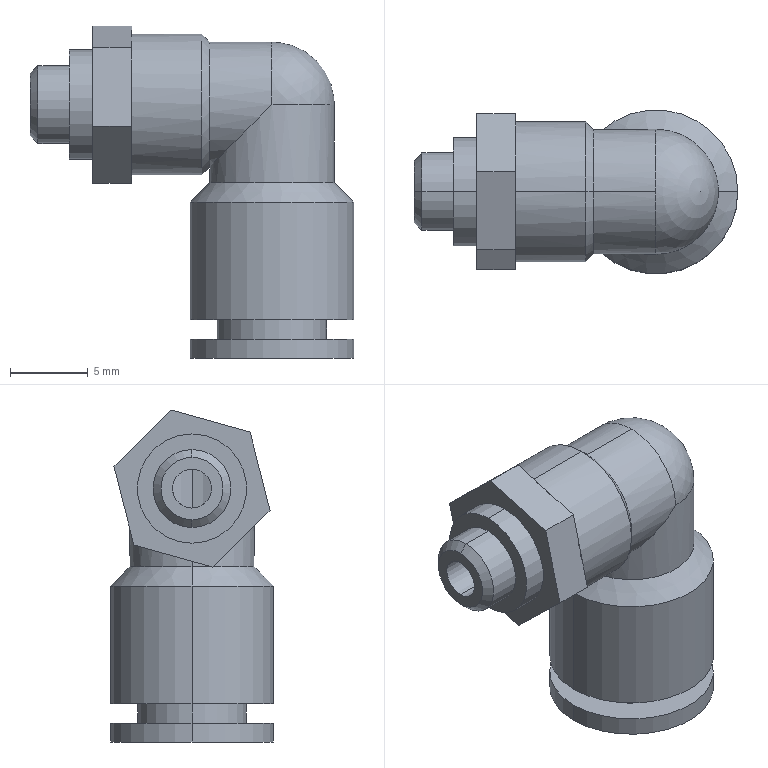Part | SolidWorks | features ICE 10, Chamfer 3, Extrusion 1, RevCut 1, Sweep 1 | 2 solids | 50 faces | box 20.75 x 10.5 x 21.285 mm | volume 1349 mm3 | cylinder 22 | plane 21 | cone 6 | sphere 1 | commonest cylinder face diameters 2.5 x4 7 x4 8 x4 10.5 x4 5 x2 6 x2
STEP:
#1=CARTESIAN_POINT('',(-4.,0.,15.));
#2=VERTEX_POINT('',#1);
#3=CARTESIAN_POINT('',(-4.,0.,17.5));
#4=VERTEX_POINT('',#3);
#5=CARTESIAN_POINT('',(-4.,0.,16.25));
#6=DIRECTION('',(-1.,0.,0.));
#7=DIRECTION('',(0.,0.,1.));
#8=AXIS2_PLACEMENT_3D('',#5,#6,#7);
#9=CIRCLE('',#8,1.25);
#10=EDGE_CURVE('',#2,#4,#9,.T.);
#11=ORIENTED_EDGE('',*,*,#10,.F.);
#12=CARTESIAN_POINT('',(-15.5,0.,15.));
#13=VERTEX_POINT('',#12);
#14=CARTESIAN_POINT('',(2.5,0.,15.));
#15=DIRECTION('',(-1.,0.,0.));
#16=VECTOR('',#15,1000.);
#17=LINE('',#14,#16);
#18=EDGE_CURVE('',#2,#13,#17,.T.);
#19=ORIENTED_EDGE('',*,*,#18,.T.);
#20=CARTESIAN_POINT('',(-15.5,0.,17.5));
#21=VERTEX_POINT('',#20);
#22=CARTESIAN_POINT('',(-15.5,0.,16.25));
#23=DIRECTION('',(-1.,0.,0.));
#24=DIRECTION('',(0.,0.,1.));
#25=AXIS2_PLACEMENT_3D('',#22,#23,#24);
#26=CIRCLE('',#25,1.25);
#27=EDGE_CURVE('',#13,#21,#26,.T.);
#28=ORIENTED_EDGE('',*,*,#27,.T.);
#29=CARTESIAN_POINT('',(2.5,0.,17.5));
#30=DIRECTION('',(-1.,0.,0.));
#31=VECTOR('',#30,1000.);
#32=LINE('',#29,#31);
#33=EDGE_CURVE('',#4,#21,#32,.T.);
#34=ORIENTED_EDGE('',*,*,#33,.F.);
#35=EDGE_LOOP('',(#11,#19,#28,#34));
#36=FACE_OUTER_BOUND('',#35,.T.);
#37=CARTESIAN_POINT('',(2.5,0.,16.25));
#38=DIRECTION('',(-1.,0.,0.));
#39=DIRECTION('',(0.,0.,1.));
#40=AXIS2_PLACEMENT_3D('',#37,#38,#39);
#41=CYLINDRICAL_SURFACE('',#40,1.25);
#42=ADVANCED_FACE('',(#36),#41,.F.);
#43=CARTESIAN_POINT('',(-15.5,0.,18.25));
#44=VERTEX_POINT('',#43);
#45=CARTESIAN_POINT('',(-15.5,0.,14.25));
#46=VERTEX_POINT('',#45);
#47=CARTESIAN_POINT('',(-15.5,0.,16.25));
#48=DIRECTION('',(-1.,0.,0.));
#49=DIRECTION('',(0.,0.,1.));
#50=AXIS2_PLACEMENT_3D('',#47,#48,#49);
#51=CIRCLE('',#50,2.);
#52=EDGE_CURVE('',#44,#46,#51,.T.);
#53=ORIENTED_EDGE('',*,*,#52,.F.);
#54=CARTESIAN_POINT('',(-15.,0.,18.75));
#55=VERTEX_POINT('',#54);
#56=CARTESIAN_POINT('',(-15.5,0.,18.25));
#57=DIRECTION('',(0.7071,0.,0.7071));
#58=VECTOR('',#57,1000.);
#59=LINE('',#56,#58);
#60=EDGE_CURVE('',#44,#55,#59,.T.);
#61=ORIENTED_EDGE('',*,*,#60,.T.);
#62=CARTESIAN_POINT('',(-15.,0.,13.75));
#63=VERTEX_POINT('',#62);
#64=CARTESIAN_POINT('',(-15.,0.,16.25));
#65=DIRECTION('',(1.,0.,0.));
#66=DIRECTION('',(0.,0.,1.));
#67=AXIS2_PLACEMENT_3D('',#64,#65,#66);
#68=CIRCLE('',#67,2.5);
#69=EDGE_CURVE('',#63,#55,#68,.T.);
#70=ORIENTED_EDGE('',*,*,#69,.F.);
#71=CARTESIAN_POINT('',(-15.5,0.,14.25));
#72=DIRECTION('',(0.7071,0.,-0.7071));
#73=VECTOR('',#72,1000.);
#74=LINE('',#71,#73);
#75=EDGE_CURVE('',#46,#63,#74,.T.);
#76=ORIENTED_EDGE('',*,*,#75,.F.);
#77=EDGE_LOOP('',(#53,#61,#70,#76));
#78=FACE_OUTER_BOUND('',#77,.T.);
#79=CARTESIAN_POINT('',(-15.5,0.,16.25));
#80=DIRECTION('',(1.,0.,0.));
#81=DIRECTION('',(0.,0.,-1.));
#82=AXIS2_PLACEMENT_3D('',#79,#80,#81);
#83=CONICAL_SURFACE('',#82,2.,0.7854);
#84=ADVANCED_FACE('',(#78),#83,.T.);
#85=ORIENTED_EDGE('',*,*,#69,.T.);
#86=CARTESIAN_POINT('',(-13.,0.,18.75));
#87=VERTEX_POINT('',#86);
#88=CARTESIAN_POINT('',(-15.5,0.,18.75));
#89=DIRECTION('',(1.,0.,0.));
#90=VECTOR('',#89,1000.);
#91=LINE('',#88,#90);
#92=EDGE_CURVE('',#55,#87,#91,.T.);
#93=ORIENTED_EDGE('',*,*,#92,.T.);
#94=CARTESIAN_POINT('',(-13.,0.,13.75));
#95=VERTEX_POINT('',#94);
#96=CARTESIAN_POINT('',(-13.,0.,16.25));
#97=DIRECTION('',(-1.,0.,0.));
#98=DIRECTION('',(0.,0.,1.));
#99=AXIS2_PLACEMENT_3D('',#96,#97,#98);
#100=CIRCLE('',#99,2.5);
#101=EDGE_CURVE('',#87,#95,#100,.T.);
#102=ORIENTED_EDGE('',*,*,#101,.T.);
#103=CARTESIAN_POINT('',(-15.5,0.,13.75));
#104=DIRECTION('',(1.,0.,0.));
#105=VECTOR('',#104,1000.);
#106=LINE('',#103,#105);
#107=EDGE_CURVE('',#63,#95,#106,.T.);
#108=ORIENTED_EDGE('',*,*,#107,.F.);
#109=EDGE_LOOP('',(#85,#93,#102,#108));
#110=FACE_OUTER_BOUND('',#109,.T.);
#111=CARTESIAN_POINT('',(-15.5,0.,16.25));
#112=DIRECTION('',(1.,0.,0.));
#113=DIRECTION('',(0.,0.,-1.));
#114=AXIS2_PLACEMENT_3D('',#111,#112,#113);
#115=CYLINDRICAL_SURFACE('',#114,2.5);
#116=ADVANCED_FACE('',(#110),#115,.T.);
#117=CARTESIAN_POINT('',(-13.,0.,19.75));
#118=VERTEX_POINT('',#117);
#119=CARTESIAN_POINT('',(-13.,0.,12.75));
#120=VERTEX_POINT('',#119);
#121=CARTESIAN_POINT('',(-13.,0.,16.25));
#122=DIRECTION('',(-1.,0.,0.));
#123=DIRECTION('',(0.,0.,1.));
#124=AXIS2_PLACEMENT_3D('',#121,#122,#123);
#125=CIRCLE('',#124,3.5);
#126=EDGE_CURVE('',#118,#120,#125,.T.);
#127=ORIENTED_EDGE('',*,*,#126,.F.);
#128=CARTESIAN_POINT('',(-11.5,0.,19.75));
#129=VERTEX_POINT('',#128);
#130=CARTESIAN_POINT('',(-13.,0.,19.75));
#131=DIRECTION('',(1.,0.,0.));
#132=VECTOR('',#131,1000.);
#133=LINE('',#130,#132);
#134=EDGE_CURVE('',#118,#129,#133,.T.);
#135=ORIENTED_EDGE('',*,*,#134,.T.);
#136=CARTESIAN_POINT('',(-11.5,0.,12.75));
#137=VERTEX_POINT('',#136);
#138=CARTESIAN_POINT('',(-11.5,0.,16.25));
#139=DIRECTION('',(-1.,0.,0.));
#140=DIRECTION('',(0.,0.,1.));
#141=AXIS2_PLACEMENT_3D('',#138,#139,#140);
#142=CIRCLE('',#141,3.5);
#143=EDGE_CURVE('',#129,#137,#142,.T.);
#144=ORIENTED_EDGE('',*,*,#143,.T.);
#145=CARTESIAN_POINT('',(-13.,0.,12.75));
#146=DIRECTION('',(1.,0.,0.));
#147=VECTOR('',#146,1000.);
#148=LINE('',#145,#147);
#149=EDGE_CURVE('',#120,#137,#148,.T.);
#150=ORIENTED_EDGE('',*,*,#149,.F.);
#151=EDGE_LOOP('',(#127,#135,#144,#150));
#152=FACE_OUTER_BOUND('',#151,.T.);
#153=CARTESIAN_POINT('',(-13.,0.,16.25));
#154=DIRECTION('',(1.,0.,0.));
#155=DIRECTION('',(0.,0.,-1.));
#156=AXIS2_PLACEMENT_3D('',#153,#154,#155);
#157=CYLINDRICAL_SURFACE('',#156,3.5);
#158=ADVANCED_FACE('',(#152),#157,.T.);
#159=CARTESIAN_POINT('',(-4.,0.,12.25));
#160=VERTEX_POINT('',#159);
#161=CARTESIAN_POINT('',(-4.,0.,20.25));
#162=VERTEX_POINT('',#161);
#163=CARTESIAN_POINT('',(-4.,0.,16.25));
#164=DIRECTION('',(1.,0.,0.));
#165=DIRECTION('',(0.,0.,1.));
#166=AXIS2_PLACEMENT_3D('',#163,#164,#165);
#167=CIRCLE('',#166,4.);
#168=EDGE_CURVE('',#160,#162,#167,.T.);
#169=ORIENTED_EDGE('',*,*,#168,.F.);
#170=CARTESIAN_POINT('',(-4.5,0.,11.75));
#171=VERTEX_POINT('',#170);
#172=CARTESIAN_POINT('',(-4.5,0.,11.75));
#173=DIRECTION('',(-0.7071,0.,-0.7071));
#174=VECTOR('',#173,1000.);
#175=LINE('',#172,#174);
#176=EDGE_CURVE('',#160,#171,#175,.T.);
#177=ORIENTED_EDGE('',*,*,#176,.T.);
#178=CARTESIAN_POINT('',(-4.5,0.,20.75));
#179=VERTEX_POINT('',#178);
#180=CARTESIAN_POINT('',(-4.5,0.,16.25));
#181=DIRECTION('',(-1.,0.,0.));
#182=DIRECTION('',(0.,0.,1.));
#183=AXIS2_PLACEMENT_3D('',#180,#181,#182);
#184=CIRCLE('',#183,4.5);
#185=EDGE_CURVE('',#179,#171,#184,.T.);
#186=ORIENTED_EDGE('',*,*,#185,.F.);
#187=CARTESIAN_POINT('',(-4.5,0.,20.75));
#188=DIRECTION('',(-0.7071,0.,0.7071));
#189=VECTOR('',#188,1000.);
#190=LINE('',#187,#189);
#191=EDGE_CURVE('',#162,#179,#190,.T.);
#192=ORIENTED_EDGE('',*,*,#191,.F.);
#193=EDGE_LOOP('',(#169,#177,#186,#192));
#194=FACE_OUTER_BOUND('',#193,.T.);
#195=CARTESIAN_POINT('',(-4.5,0.,16.25));
#196=DIRECTION('',(-1.,0.,0.));
#197=DIRECTION('',(0.,0.,1.));
#198=AXIS2_PLACEMENT_3D('',#195,#196,#197);
#199=CONICAL_SURFACE('',#198,4.5,0.7854);
#200=ADVANCED_FACE('',(#194),#199,.T.);
#201=CARTESIAN_POINT('',(-9.,0.,20.75));
#202=VERTEX_POINT('',#201);
#203=CARTESIAN_POINT('',(-9.,3.143,19.47));
#204=VERTEX_POINT('',#203);
#205=CARTESIAN_POINT('',(-9.,0.,16.25));
#206=DIRECTION('',(-1.,0.,0.));
#207=DIRECTION('',(0.,0.,1.));
#208=AXIS2_PLACEMENT_3D('',#205,#206,#207);
#209=CIRCLE('',#208,4.5);
#210=EDGE_CURVE('',#202,#204,#209,.T.);
#211=ORIENTED_EDGE('',*,*,#210,.F.);
#212=CARTESIAN_POINT('',(-9.,0.,20.75));
#213=DIRECTION('',(1.,0.,0.));
#214=VECTOR('',#213,1000.);
#215=LINE('',#212,#214);
#216=EDGE_CURVE('',#202,#179,#215,.T.);
#217=ORIENTED_EDGE('',*,*,#216,.T.);
#218=ORIENTED_EDGE('',*,*,#185,.T.);
#219=CARTESIAN_POINT('',(-9.,0.,11.75));
#220=VERTEX_POINT('',#219);
#221=CARTESIAN_POINT('',(-9.,0.,11.75));
#222=DIRECTION('',(1.,0.,0.));
#223=VECTOR('',#222,1000.);
#224=LINE('',#221,#223);
#225=EDGE_CURVE('',#220,#171,#224,.T.);
#226=ORIENTED_EDGE('',*,*,#225,.F.);
#227=CARTESIAN_POINT('',(-9.,1.217,11.918));
#228=VERTEX_POINT('',#227);
#229=CARTESIAN_POINT('',(-9.,0.,16.25));
#230=DIRECTION('',(-1.,0.,0.));
#231=DIRECTION('',(0.,0.,1.));
#232=AXIS2_PLACEMENT_3D('',#229,#230,#231);
#233=CIRCLE('',#232,4.5);
#234=EDGE_CURVE('',#228,#220,#233,.T.);
#235=ORIENTED_EDGE('',*,*,#234,.F.);
#236=CARTESIAN_POINT('',(-9.,4.36,15.138));
#237=VERTEX_POINT('',#236);
#238=CARTESIAN_POINT('',(-9.,0.,16.25));
#239=DIRECTION('',(-1.,0.,0.));
#240=DIRECTION('',(0.,0.,1.));
#241=AXIS2_PLACEMENT_3D('',#238,#239,#240);
#242=CIRCLE('',#241,4.5);
#243=EDGE_CURVE('',#237,#228,#242,.T.);
#244=ORIENTED_EDGE('',*,*,#243,.F.);
#245=CARTESIAN_POINT('',(-9.,0.,16.25));
#246=DIRECTION('',(-1.,0.,0.));
#247=DIRECTION('',(0.,0.,1.));
#248=AXIS2_PLACEMENT_3D('',#245,#246,#247);
#249=CIRCLE('',#248,4.5);
#250=EDGE_CURVE('',#204,#237,#249,.T.);
#251=ORIENTED_EDGE('',*,*,#250,.F.);
#252=EDGE_LOOP('',(#211,#217,#218,#226,#235,#244,#251));
#253=FACE_OUTER_BOUND('',#252,.T.);
#254=CARTESIAN_POINT('',(-9.,0.,16.25));
#255=DIRECTION('',(1.,0.,0.));
#256=DIRECTION('',(0.,0.,-1.));
#257=AXIS2_PLACEMENT_3D('',#254,#255,#256);
#258=CYLINDRICAL_SURFACE('',#257,4.5);
#259=ADVANCED_FACE('',(#253),#258,.T.);
#260=CARTESIAN_POINT('',(-13.,0.,16.25));
#261=DIRECTION('',(-1.,0.,0.));
#262=DIRECTION('',(0.,0.,1.));
#263=AXIS2_PLACEMENT_3D('',#260,#261,#262);
#264=CIRCLE('',#263,3.5);
#265=EDGE_CURVE('',#120,#118,#264,.T.);
#266=ORIENTED_EDGE('',*,*,#265,.T.);
#267=ORIENTED_EDGE('',*,*,#126,.T.);
#268=EDGE_LOOP('',(#266,#267));
#269=FACE_OUTER_BOUND('',#268,.T.);
#270=CARTESIAN_POINT('',(-13.,0.,16.25));
#271=DIRECTION('',(-1.,0.,0.));
#272=DIRECTION('',(0.,0.,1.));
#273=AXIS2_PLACEMENT_3D('',#270,#271,#272);
#274=CIRCLE('',#273,2.5);
#275=EDGE_CURVE('',#95,#87,#274,.T.);
#276=ORIENTED_EDGE('',*,*,#275,.F.);
#277=ORIENTED_EDGE('',*,*,#101,.F.);
#278=EDGE_LOOP('',(#276,#277));
#279=FACE_BOUND('',#278,.T.);
#280=CARTESIAN_POINT('',(-13.,0.,16.25));
#281=DIRECTION('',(-1.,0.,0.));
#282=DIRECTION('',(0.,0.,1.));
#283=AXIS2_PLACEMENT_3D('',#280,#281,#282);
#284=PLANE('',#283);
#285=ADVANCED_FACE('',(#269,#279),#284,.T.);
#286=CARTESIAN_POINT('',(-11.5,-3.718,19.88));
#287=VERTEX_POINT('',#286);
#288=CARTESIAN_POINT('',(-11.5,1.284,21.285));
#289=VERTEX_POINT('',#288);
#290=CARTESIAN_POINT('',(-11.5,-3.718,19.88));
#291=DIRECTION('',(0.,0.9627,0.2704));
#292=VECTOR('',#291,1000.);
#293=LINE('',#290,#292);
#294=EDGE_CURVE('',#287,#289,#293,.T.);
#295=ORIENTED_EDGE('',*,*,#294,.T.);
#296=CARTESIAN_POINT('',(-11.5,5.003,17.655));
#297=VERTEX_POINT('',#296);
#298=CARTESIAN_POINT('',(-11.5,1.284,21.285));
#299=DIRECTION('',(0.,0.7156,-0.6985));
#300=VECTOR('',#299,1000.);
#301=LINE('',#298,#300);
#302=EDGE_CURVE('',#289,#297,#301,.T.);
#303=ORIENTED_EDGE('',*,*,#302,.T.);
#304=CARTESIAN_POINT('',(-11.5,3.718,12.62));
#305=VERTEX_POINT('',#304);
#306=CARTESIAN_POINT('',(-11.5,5.003,17.655));
#307=DIRECTION('',(0.,-0.2472,-0.969));
#308=VECTOR('',#307,1000.);
#309=LINE('',#306,#308);
#310=EDGE_CURVE('',#297,#305,#309,.T.);
#311=ORIENTED_EDGE('',*,*,#310,.T.);
#312=CARTESIAN_POINT('',(-11.5,-1.284,11.215));
#313=VERTEX_POINT('',#312);
#314=CARTESIAN_POINT('',(-11.5,3.718,12.62));
#315=DIRECTION('',(0.,-0.9627,-0.2704));
#316=VECTOR('',#315,1000.);
#317=LINE('',#314,#316);
#318=EDGE_CURVE('',#305,#313,#317,.T.);
#319=ORIENTED_EDGE('',*,*,#318,.T.);
#320=CARTESIAN_POINT('',(-11.5,-5.003,14.845));
#321=VERTEX_POINT('',#320);
#322=CARTESIAN_POINT('',(-11.5,-1.284,11.215));
#323=DIRECTION('',(0.,-0.7156,0.6985));
#324=VECTOR('',#323,1000.);
#325=LINE('',#322,#324);
#326=EDGE_CURVE('',#313,#321,#325,.T.);
#327=ORIENTED_EDGE('',*,*,#326,.T.);
#328=CARTESIAN_POINT('',(-11.5,-5.003,14.845));
#329=DIRECTION('',(0.,0.2472,0.969));
#330=VECTOR('',#329,1000.);
#331=LINE('',#328,#330);
#332=EDGE_CURVE('',#321,#287,#331,.T.);
#333=ORIENTED_EDGE('',*,*,#332,.T.);
#334=EDGE_LOOP('',(#295,#303,#311,#319,#327,#333));
#335=FACE_OUTER_BOUND('',#334,.T.);
#336=CARTESIAN_POINT('',(-11.5,0.,16.25));
#337=DIRECTION('',(-1.,0.,0.));
#338=DIRECTION('',(0.,0.,1.));
#339=AXIS2_PLACEMENT_3D('',#336,#337,#338);
#340=CIRCLE('',#339,3.5);
#341=EDGE_CURVE('',#137,#129,#340,.T.);
#342=ORIENTED_EDGE('',*,*,#341,.F.);
#343=ORIENTED_EDGE('',*,*,#143,.F.);
#344=EDGE_LOOP('',(#342,#343));
#345=FACE_BOUND('',#344,.T.);
#346=CARTESIAN_POINT('',(-11.5,0.,0.));
#347=DIRECTION('',(-1.,0.,0.));
#348=DIRECTION('',(0.,0.,1.));
#349=AXIS2_PLACEMENT_3D('',#346,#347,#348);
#350=PLANE('',#349);
#351=ADVANCED_FACE('',(#335,#345),#350,.T.);
#352=ORIENTED_EDGE('',*,*,#216,.F.);
#353=CARTESIAN_POINT('',(-9.,-1.217,20.582));
#354=VERTEX_POINT('',#353);
#355=CARTESIAN_POINT('',(-9.,0.,16.25));
#356=DIRECTION('',(-1.,0.,0.));
#357=DIRECTION('',(0.,0.,1.));
#358=AXIS2_PLACEMENT_3D('',#355,#356,#357);
#359=CIRCLE('',#358,4.5);
#360=EDGE_CURVE('',#354,#202,#359,.T.);
#361=ORIENTED_EDGE('',*,*,#360,.F.);
#362=CARTESIAN_POINT('',(-9.,-4.36,17.362));
#363=VERTEX_POINT('',#362);
#364=CARTESIAN_POINT('',(-9.,0.,16.25));
#365=DIRECTION('',(-1.,0.,0.));
#366=DIRECTION('',(0.,0.,1.));
#367=AXIS2_PLACEMENT_3D('',#364,#365,#366);
#368=CIRCLE('',#367,4.5);
#369=EDGE_CURVE('',#363,#354,#368,.T.);
#370=ORIENTED_EDGE('',*,*,#369,.F.);
#371=CARTESIAN_POINT('',(-9.,-3.143,13.03));
#372=VERTEX_POINT('',#371);
#373=CARTESIAN_POINT('',(-9.,0.,16.25));
#374=DIRECTION('',(-1.,0.,0.));
#375=DIRECTION('',(0.,0.,1.));
#376=AXIS2_PLACEMENT_3D('',#373,#374,#375);
#377=CIRCLE('',#376,4.5);
#378=EDGE_CURVE('',#372,#363,#377,.T.);
#379=ORIENTED_EDGE('',*,*,#378,.F.);
#380=CARTESIAN_POINT('',(-9.,0.,16.25));
#381=DIRECTION('',(-1.,0.,0.));
#382=DIRECTION('',(0.,0.,1.));
#383=AXIS2_PLACEMENT_3D('',#380,#381,#382);
#384=CIRCLE('',#383,4.5);
#385=EDGE_CURVE('',#220,#372,#384,.T.);
#386=ORIENTED_EDGE('',*,*,#385,.F.);
#387=ORIENTED_EDGE('',*,*,#225,.T.);
#388=CARTESIAN_POINT('',(-4.5,0.,16.25));
#389=DIRECTION('',(-1.,0.,0.));
#390=DIRECTION('',(0.,0.,1.));
#391=AXIS2_PLACEMENT_3D('',#388,#389,#390);
#392=CIRCLE('',#391,4.5);
#393=EDGE_CURVE('',#171,#179,#392,.T.);
#394=ORIENTED_EDGE('',*,*,#393,.T.);
#395=EDGE_LOOP('',(#352,#361,#370,#379,#386,#387,#394));
#396=FACE_OUTER_BOUND('',#395,.T.);
#397=CARTESIAN_POINT('',(-9.,0.,16.25));
#398=DIRECTION('',(1.,0.,0.));
#399=DIRECTION('',(0.,0.,-1.));
#400=AXIS2_PLACEMENT_3D('',#397,#398,#399);
#401=CYLINDRICAL_SURFACE('',#400,4.5);
#402=ADVANCED_FACE('',(#396),#401,.T.);
#403=CARTESIAN_POINT('',(-4.,0.,16.25));
#404=DIRECTION('',(-1.,0.,0.));
#405=DIRECTION('',(0.,0.,1.));
#406=AXIS2_PLACEMENT_3D('',#403,#404,#405);
#407=CIRCLE('',#406,1.25);
#408=EDGE_CURVE('',#4,#2,#407,.T.);
#409=ORIENTED_EDGE('',*,*,#408,.T.);
#410=ORIENTED_EDGE('',*,*,#10,.T.);
#411=EDGE_LOOP('',(#409,#410));
#412=FACE_BOUND('',#411,.T.);
#413=CARTESIAN_POINT('',(-4.,0.,16.25));
#414=DIRECTION('',(1.,0.,0.));
#415=DIRECTION('',(0.,0.,1.));
#416=AXIS2_PLACEMENT_3D('',#413,#414,#415);
#417=CIRCLE('',#416,4.);
#418=EDGE_CURVE('',#162,#160,#417,.T.);
#419=ORIENTED_EDGE('',*,*,#418,.T.);
#420=ORIENTED_EDGE('',*,*,#168,.T.);
#421=EDGE_LOOP('',(#419,#420));
#422=FACE_OUTER_BOUND('',#421,.T.);
#423=CARTESIAN_POINT('',(-4.,0.,16.25));
#424=DIRECTION('',(-1.,0.,0.));
#425=DIRECTION('',(0.,0.,1.));
#426=AXIS2_PLACEMENT_3D('',#423,#424,#425);
#427=PLANE('',#426);
#428=ADVANCED_FACE('',(#412,#422),#427,.F.);
#429=ORIENTED_EDGE('',*,*,#176,.F.);
#430=ORIENTED_EDGE('',*,*,#418,.F.);
#431=ORIENTED_EDGE('',*,*,#191,.T.);
#432=ORIENTED_EDGE('',*,*,#393,.F.);
#433=EDGE_LOOP('',(#429,#430,#431,#432));
#434=FACE_OUTER_BOUND('',#433,.T.);
#435=CARTESIAN_POINT('',(-4.5,0.,16.25));
#436=DIRECTION('',(-1.,0.,0.));
#437=DIRECTION('',(0.,0.,1.));
#438=AXIS2_PLACEMENT_3D('',#435,#436,#437);
#439=CONICAL_SURFACE('',#438,4.5,0.7854);
#440=ADVANCED_FACE('',(#434),#439,.T.);
#441=CARTESIAN_POINT('',(-9.,5.003,17.655));
#442=VERTEX_POINT('',#441);
#443=CARTESIAN_POINT('',(-9.,1.284,21.285));
#444=DIRECTION('',(0.,0.7156,-0.6985));
#445=VECTOR('',#444,1000.);
#446=LINE('',#443,#445);
#447=EDGE_CURVE('',#204,#442,#446,.T.);
#448=ORIENTED_EDGE('',*,*,#447,.F.);
#449=ORIENTED_EDGE('',*,*,#250,.T.);
#450=CARTESIAN_POINT('',(-9.,5.003,17.655));
#451=DIRECTION('',(0.,-0.2472,-0.969));
#452=VECTOR('',#451,1000.);
#453=LINE('',#450,#452);
#454=EDGE_CURVE('',#442,#237,#453,.T.);
#455=ORIENTED_EDGE('',*,*,#454,.F.);
#456=EDGE_LOOP('',(#448,#449,#455));
#457=FACE_OUTER_BOUND('',#456,.T.);
#458=CARTESIAN_POINT('',(-9.,0.,0.));
#459=DIRECTION('',(-1.,0.,0.));
#460=DIRECTION('',(0.,0.,1.));
#461=AXIS2_PLACEMENT_3D('',#458,#459,#460);
#462=PLANE('',#461);
#463=ADVANCED_FACE('',(#457),#462,.F.);
#464=CARTESIAN_POINT('',(-9.,3.718,12.62));
#465=VERTEX_POINT('',#464);
#466=CARTESIAN_POINT('',(-9.,5.003,17.655));
#467=DIRECTION('',(0.,-0.2472,-0.969));
#468=VECTOR('',#467,1000.);
#469=LINE('',#466,#468);
#470=EDGE_CURVE('',#237,#465,#469,.T.);
#471=ORIENTED_EDGE('',*,*,#470,.F.);
#472=ORIENTED_EDGE('',*,*,#243,.T.);
#473=CARTESIAN_POINT('',(-9.,3.718,12.62));
#474=DIRECTION('',(0.,-0.9627,-0.2704));
#475=VECTOR('',#474,1000.);
#476=LINE('',#473,#475);
#477=EDGE_CURVE('',#465,#228,#476,.T.);
#478=ORIENTED_EDGE('',*,*,#477,.F.);
#479=EDGE_LOOP('',(#471,#472,#478));
#480=FACE_OUTER_BOUND('',#479,.T.);
#481=CARTESIAN_POINT('',(-9.,0.,0.));
#482=DIRECTION('',(-1.,0.,0.));
#483=DIRECTION('',(0.,0.,1.));
#484=AXIS2_PLACEMENT_3D('',#481,#482,#483);
#485=PLANE('',#484);
#486=ADVANCED_FACE('',(#480),#485,.F.);
#487=CARTESIAN_POINT('',(-9.,-1.284,11.215));
#488=VERTEX_POINT('',#487);
#489=CARTESIAN_POINT('',(-9.,3.718,12.62));
#490=DIRECTION('',(0.,-0.9627,-0.2704));
#491=VECTOR('',#490,1000.);
#492=LINE('',#489,#491);
#493=EDGE_CURVE('',#228,#488,#492,.T.);
#494=ORIENTED_EDGE('',*,*,#493,.F.);
#495=ORIENTED_EDGE('',*,*,#234,.T.);
#496=ORIENTED_EDGE('',*,*,#385,.T.);
#497=CARTESIAN_POINT('',(-9.,-1.284,11.215));
#498=DIRECTION('',(0.,-0.7156,0.6985));
#499=VECTOR('',#498,1000.);
#500=LINE('',#497,#499);
#501=EDGE_CURVE('',#488,#372,#500,.T.);
#502=ORIENTED_EDGE('',*,*,#501,.F.);
#503=EDGE_LOOP('',(#494,#495,#496,#502));
#504=FACE_OUTER_BOUND('',#503,.T.);
#505=CARTESIAN_POINT('',(-9.,0.,0.));
#506=DIRECTION('',(-1.,0.,0.));
#507=DIRECTION('',(0.,0.,1.));
#508=AXIS2_PLACEMENT_3D('',#505,#506,#507);
#509=PLANE('',#508);
#510=ADVANCED_FACE('',(#504),#509,.F.);
#511=CARTESIAN_POINT('',(-9.,-5.003,14.845));
#512=VERTEX_POINT('',#511);
#513=CARTESIAN_POINT('',(-9.,-1.284,11.215));
#514=DIRECTION('',(0.,-0.7156,0.6985));
#515=VECTOR('',#514,1000.);
#516=LINE('',#513,#515);
#517=EDGE_CURVE('',#372,#512,#516,.T.);
#518=ORIENTED_EDGE('',*,*,#517,.F.);
#519=ORIENTED_EDGE('',*,*,#378,.T.);
#520=CARTESIAN_POINT('',(-9.,-5.003,14.845));
#521=DIRECTION('',(0.,0.2472,0.969));
#522=VECTOR('',#521,1000.);
#523=LINE('',#520,#522);
#524=EDGE_CURVE('',#512,#363,#523,.T.);
#525=ORIENTED_EDGE('',*,*,#524,.F.);
#526=EDGE_LOOP('',(#518,#519,#525));
#527=FACE_OUTER_BOUND('',#526,.T.);
#528=CARTESIAN_POINT('',(-9.,0.,0.));
#529=DIRECTION('',(-1.,0.,0.));
#530=DIRECTION('',(0.,0.,1.));
#531=AXIS2_PLACEMENT_3D('',#528,#529,#530);
#532=PLANE('',#531);
#533=ADVANCED_FACE('',(#527),#532,.F.);
#534=CARTESIAN_POINT('',(-9.,-3.718,19.88));
#535=VERTEX_POINT('',#534);
#536=CARTESIAN_POINT('',(-9.,-5.003,14.845));
#537=DIRECTION('',(0.,0.2472,0.969));
#538=VECTOR('',#537,1000.);
#539=LINE('',#536,#538);
#540=EDGE_CURVE('',#363,#535,#539,.T.);
#541=ORIENTED_EDGE('',*,*,#540,.F.);
#542=ORIENTED_EDGE('',*,*,#369,.T.);
#543=CARTESIAN_POINT('',(-9.,-3.718,19.88));
#544=DIRECTION('',(0.,0.9627,0.2704));
#545=VECTOR('',#544,1000.);
#546=LINE('',#543,#545);
#547=EDGE_CURVE('',#535,#354,#546,.T.);
#548=ORIENTED_EDGE('',*,*,#547,.F.);
#549=EDGE_LOOP('',(#541,#542,#548));
#550=FACE_OUTER_BOUND('',#549,.T.);
#551=CARTESIAN_POINT('',(-9.,0.,0.));
#552=DIRECTION('',(-1.,0.,0.));
#553=DIRECTION('',(0.,0.,1.));
#554=AXIS2_PLACEMENT_3D('',#551,#552,#553);
#555=PLANE('',#554);
#556=ADVANCED_FACE('',(#550),#555,.F.);
#557=CARTESIAN_POINT('',(-9.,1.284,21.285));
#558=VERTEX_POINT('',#557);
#559=CARTESIAN_POINT('',(-9.,-3.718,19.88));
#560=DIRECTION('',(0.,0.9627,0.2704));
#561=VECTOR('',#560,1000.);
#562=LINE('',#559,#561);
#563=EDGE_CURVE('',#354,#558,#562,.T.);
#564=ORIENTED_EDGE('',*,*,#563,.F.);
#565=ORIENTED_EDGE('',*,*,#360,.T.);
#566=ORIENTED_EDGE('',*,*,#210,.T.);
#567=CARTESIAN_POINT('',(-9.,1.284,21.285));
#568=DIRECTION('',(0.,0.7156,-0.6985));
#569=VECTOR('',#568,1000.);
#570=LINE('',#567,#569);
#571=EDGE_CURVE('',#558,#204,#570,.T.);
#572=ORIENTED_EDGE('',*,*,#571,.F.);
#573=EDGE_LOOP('',(#564,#565,#566,#572));
#574=FACE_OUTER_BOUND('',#573,.T.);
#575=CARTESIAN_POINT('',(-9.,0.,0.));
#576=DIRECTION('',(-1.,0.,0.));
#577=DIRECTION('',(0.,0.,1.));
#578=AXIS2_PLACEMENT_3D('',#575,#576,#577);
#579=PLANE('',#578);
#580=ADVANCED_FACE('',(#574),#579,.F.);
#581=ORIENTED_EDGE('',*,*,#547,.T.);
#582=ORIENTED_EDGE('',*,*,#563,.T.);
#583=CARTESIAN_POINT('',(-11.5,1.284,21.285));
#584=DIRECTION('',(1.,0.,0.));
#585=VECTOR('',#584,1000.);
#586=LINE('',#583,#585);
#587=EDGE_CURVE('',#289,#558,#586,.T.);
#588=ORIENTED_EDGE('',*,*,#587,.F.);
#589=ORIENTED_EDGE('',*,*,#294,.F.);
#590=CARTESIAN_POINT('',(-11.5,-3.718,19.88));
#591=DIRECTION('',(1.,0.,0.));
#592=VECTOR('',#591,1000.);
#593=LINE('',#590,#592);
#594=EDGE_CURVE('',#287,#535,#593,.T.);
#595=ORIENTED_EDGE('',*,*,#594,.T.);
#596=EDGE_LOOP('',(#581,#582,#588,#589,#595));
#597=FACE_OUTER_BOUND('',#596,.T.);
#598=CARTESIAN_POINT('',(-11.5,-3.718,19.88));
#599=DIRECTION('',(0.,0.2704,-0.9627));
#600=DIRECTION('',(0.,0.9627,0.2704));
#601=AXIS2_PLACEMENT_3D('',#598,#599,#600);
#602=PLANE('',#601);
#603=ADVANCED_FACE('',(#597),#602,.F.);
#604=ORIENTED_EDGE('',*,*,#571,.T.);
#605=ORIENTED_EDGE('',*,*,#447,.T.);
#606=CARTESIAN_POINT('',(-11.5,5.003,17.655));
#607=DIRECTION('',(1.,0.,0.));
#608=VECTOR('',#607,1000.);
#609=LINE('',#606,#608);
#610=EDGE_CURVE('',#297,#442,#609,.T.);
#611=ORIENTED_EDGE('',*,*,#610,.F.);
#612=ORIENTED_EDGE('',*,*,#302,.F.);
#613=ORIENTED_EDGE('',*,*,#587,.T.);
#614=EDGE_LOOP('',(#604,#605,#611,#612,#613));
#615=FACE_OUTER_BOUND('',#614,.T.);
#616=CARTESIAN_POINT('',(-11.5,1.284,21.285));
#617=DIRECTION('',(0.,-0.6985,-0.7156));
#618=DIRECTION('',(0.,0.7156,-0.6985));
#619=AXIS2_PLACEMENT_3D('',#616,#617,#618);
#620=PLANE('',#619);
#621=ADVANCED_FACE('',(#615),#620,.F.);
#622=ORIENTED_EDGE('',*,*,#454,.T.);
#623=ORIENTED_EDGE('',*,*,#470,.T.);
#624=CARTESIAN_POINT('',(-11.5,3.718,12.62));
#625=DIRECTION('',(1.,0.,0.));
#626=VECTOR('',#625,1000.);
#627=LINE('',#624,#626);
#628=EDGE_CURVE('',#305,#465,#627,.T.);
#629=ORIENTED_EDGE('',*,*,#628,.F.);
#630=ORIENTED_EDGE('',*,*,#310,.F.);
#631=ORIENTED_EDGE('',*,*,#610,.T.);
#632=EDGE_LOOP('',(#622,#623,#629,#630,#631));
#633=FACE_OUTER_BOUND('',#632,.T.);
#634=CARTESIAN_POINT('',(-11.5,5.003,17.655));
#635=DIRECTION('',(0.,-0.969,0.2472));
#636=DIRECTION('',(0.,-0.2472,-0.969));
#637=AXIS2_PLACEMENT_3D('',#634,#635,#636);
#638=PLANE('',#637);
#639=ADVANCED_FACE('',(#633),#638,.F.);
#640=ORIENTED_EDGE('',*,*,#477,.T.);
#641=ORIENTED_EDGE('',*,*,#493,.T.);
#642=CARTESIAN_POINT('',(-11.5,-1.284,11.215));
#643=DIRECTION('',(1.,0.,0.));
#644=VECTOR('',#643,1000.);
#645=LINE('',#642,#644);
#646=EDGE_CURVE('',#313,#488,#645,.T.);
#647=ORIENTED_EDGE('',*,*,#646,.F.);
#648=ORIENTED_EDGE('',*,*,#318,.F.);
#649=ORIENTED_EDGE('',*,*,#628,.T.);
#650=EDGE_LOOP('',(#640,#641,#647,#648,#649));
#651=FACE_OUTER_BOUND('',#650,.T.);
#652=CARTESIAN_POINT('',(-11.5,3.718,12.62));
#653=DIRECTION('',(0.,-0.2704,0.9627));
#654=DIRECTION('',(0.,-0.9627,-0.2704));
#655=AXIS2_PLACEMENT_3D('',#652,#653,#654);
#656=PLANE('',#655);
#657=ADVANCED_FACE('',(#651),#656,.F.);
#658=ORIENTED_EDGE('',*,*,#501,.T.);
#659=ORIENTED_EDGE('',*,*,#517,.T.);
#660=CARTESIAN_POINT('',(-11.5,-5.003,14.845));
#661=DIRECTION('',(1.,0.,0.));
#662=VECTOR('',#661,1000.);
#663=LINE('',#660,#662);
#664=EDGE_CURVE('',#321,#512,#663,.T.);
#665=ORIENTED_EDGE('',*,*,#664,.F.);
#666=ORIENTED_EDGE('',*,*,#326,.F.);
#667=ORIENTED_EDGE('',*,*,#646,.T.);
#668=EDGE_LOOP('',(#658,#659,#665,#666,#667));
#669=FACE_OUTER_BOUND('',#668,.T.);
#670=CARTESIAN_POINT('',(-11.5,-1.284,11.215));
#671=DIRECTION('',(0.,0.6985,0.7156));
#672=DIRECTION('',(0.,-0.7156,0.6985));
#673=AXIS2_PLACEMENT_3D('',#670,#671,#672);
#674=PLANE('',#673);
#675=ADVANCED_FACE('',(#669),#674,.F.);
#676=ORIENTED_EDGE('',*,*,#524,.T.);
#677=ORIENTED_EDGE('',*,*,#540,.T.);
#678=ORIENTED_EDGE('',*,*,#594,.F.);
#679=ORIENTED_EDGE('',*,*,#332,.F.);
#680=ORIENTED_EDGE('',*,*,#664,.T.);
#681=EDGE_LOOP('',(#676,#677,#678,#679,#680));
#682=FACE_OUTER_BOUND('',#681,.T.);
#683=CARTESIAN_POINT('',(-11.5,-5.003,14.845));
#684=DIRECTION('',(0.,0.969,-0.2472));
#685=DIRECTION('',(0.,0.2472,0.969));
#686=AXIS2_PLACEMENT_3D('',#683,#684,#685);
#687=PLANE('',#686);
#688=ADVANCED_FACE('',(#682),#687,.F.);
#689=ORIENTED_EDGE('',*,*,#134,.F.);
#690=ORIENTED_EDGE('',*,*,#265,.F.);
#691=ORIENTED_EDGE('',*,*,#149,.T.);
#692=ORIENTED_EDGE('',*,*,#341,.T.);
#693=EDGE_LOOP('',(#689,#690,#691,#692));
#694=FACE_OUTER_BOUND('',#693,.T.);
#695=CARTESIAN_POINT('',(-13.,0.,16.25));
#696=DIRECTION('',(1.,0.,0.));
#697=DIRECTION('',(0.,0.,-1.));
#698=AXIS2_PLACEMENT_3D('',#695,#696,#697);
#699=CYLINDRICAL_SURFACE('',#698,3.5);
#700=ADVANCED_FACE('',(#694),#699,.T.);
#701=ORIENTED_EDGE('',*,*,#92,.F.);
#702=CARTESIAN_POINT('',(-15.,0.,16.25));
#703=DIRECTION('',(1.,0.,0.));
#704=DIRECTION('',(0.,0.,1.));
#705=AXIS2_PLACEMENT_3D('',#702,#703,#704);
#706=CIRCLE('',#705,2.5);
#707=EDGE_CURVE('',#55,#63,#706,.T.);
#708=ORIENTED_EDGE('',*,*,#707,.T.);
#709=ORIENTED_EDGE('',*,*,#107,.T.);
#710=ORIENTED_EDGE('',*,*,#275,.T.);
#711=EDGE_LOOP('',(#701,#708,#709,#710));
#712=FACE_OUTER_BOUND('',#711,.T.);
#713=CARTESIAN_POINT('',(-15.5,0.,16.25));
#714=DIRECTION('',(1.,0.,0.));
#715=DIRECTION('',(0.,0.,-1.));
#716=AXIS2_PLACEMENT_3D('',#713,#714,#715);
#717=CYLINDRICAL_SURFACE('',#716,2.5);
#718=ADVANCED_FACE('',(#712),#717,.T.);
#719=CARTESIAN_POINT('',(-15.5,0.,16.25));
#720=DIRECTION('',(-1.,0.,0.));
#721=DIRECTION('',(0.,0.,1.));
#722=AXIS2_PLACEMENT_3D('',#719,#720,#721);
#723=CIRCLE('',#722,1.25);
#724=EDGE_CURVE('',#21,#13,#723,.T.);
#725=ORIENTED_EDGE('',*,*,#724,.F.);
#726=ORIENTED_EDGE('',*,*,#27,.F.);
#727=EDGE_LOOP('',(#725,#726));
#728=FACE_BOUND('',#727,.T.);
#729=CARTESIAN_POINT('',(-15.5,0.,16.25));
#730=DIRECTION('',(-1.,0.,0.));
#731=DIRECTION('',(0.,0.,1.));
#732=AXIS2_PLACEMENT_3D('',#729,#730,#731);
#733=CIRCLE('',#732,2.);
#734=EDGE_CURVE('',#46,#44,#733,.T.);
#735=ORIENTED_EDGE('',*,*,#734,.T.);
#736=ORIENTED_EDGE('',*,*,#52,.T.);
#737=EDGE_LOOP('',(#735,#736));
#738=FACE_OUTER_BOUND('',#737,.T.);
#739=CARTESIAN_POINT('',(-15.5,0.,16.25));
#740=DIRECTION('',(-1.,0.,0.));
#741=DIRECTION('',(0.,0.,1.));
#742=AXIS2_PLACEMENT_3D('',#739,#740,#741);
#743=PLANE('',#742);
#744=ADVANCED_FACE('',(#728,#738),#743,.T.);
#745=ORIENTED_EDGE('',*,*,#60,.F.);
#746=ORIENTED_EDGE('',*,*,#734,.F.);
#747=ORIENTED_EDGE('',*,*,#75,.T.);
#748=ORIENTED_EDGE('',*,*,#707,.F.);
#749=EDGE_LOOP('',(#745,#746,#747,#748));
#750=FACE_OUTER_BOUND('',#749,.T.);
#751=CARTESIAN_POINT('',(-15.5,0.,16.25));
#752=DIRECTION('',(1.,0.,0.));
#753=DIRECTION('',(0.,0.,-1.));
#754=AXIS2_PLACEMENT_3D('',#751,#752,#753);
#755=CONICAL_SURFACE('',#754,2.,0.7854);
#756=ADVANCED_FACE('',(#750),#755,.T.);
#757=ORIENTED_EDGE('',*,*,#18,.F.);
#758=ORIENTED_EDGE('',*,*,#408,.F.);
#759=ORIENTED_EDGE('',*,*,#33,.T.);
#760=ORIENTED_EDGE('',*,*,#724,.T.);
#761=EDGE_LOOP('',(#757,#758,#759,#760));
#762=FACE_OUTER_BOUND('',#761,.T.);
#763=CARTESIAN_POINT('',(2.5,0.,16.25));
#764=DIRECTION('',(-1.,0.,0.));
#765=DIRECTION('',(0.,0.,1.));
#766=AXIS2_PLACEMENT_3D('',#763,#764,#765);
#767=CYLINDRICAL_SURFACE('',#766,1.25);
#768=ADVANCED_FACE('',(#762),#767,.F.);
#769=CLOSED_SHELL('',(#42,#84,#116,#158,#200,#259,#285,#351,#402,#428,#440,#463,#486,#510,#533,#556,#580,#603,#621,#639,#657,#675,#688,#700,#718,#744,#756,#768));
#770=MANIFOLD_SOLID_BREP('',#769);
#771=CARTESIAN_POINT('',(3.,0.,18.));
#772=VERTEX_POINT('',#771);
#773=CARTESIAN_POINT('',(-3.,0.,18.));
#774=VERTEX_POINT('',#773);
#775=CARTESIAN_POINT('',(0.,0.,18.));
#776=DIRECTION('',(0.,0.,-1.));
#777=DIRECTION('',(-1.,0.,0.));
#778=AXIS2_PLACEMENT_3D('',#775,#776,#777);
#779=CIRCLE('',#778,3.);
#780=EDGE_CURVE('',#772,#774,#779,.T.);
#781=ORIENTED_EDGE('',*,*,#780,.F.);
#782=CARTESIAN_POINT('',(3.,0.,0.));
#783=VERTEX_POINT('',#782);
#784=CARTESIAN_POINT('',(3.,0.,18.));
#785=DIRECTION('',(0.,0.,-1.));
#786=VECTOR('',#785,1000.);
#787=LINE('',#784,#786);
#788=EDGE_CURVE('',#772,#783,#787,.T.);
#789=ORIENTED_EDGE('',*,*,#788,.T.);
#790=CARTESIAN_POINT('',(-3.,0.,0.));
#791=VERTEX_POINT('',#790);
#792=CARTESIAN_POINT('',(0.,0.,0.));
#793=DIRECTION('',(0.,0.,-1.));
#794=DIRECTION('',(-1.,0.,0.));
#795=AXIS2_PLACEMENT_3D('',#792,#793,#794);
#796=CIRCLE('',#795,3.);
#797=EDGE_CURVE('',#783,#791,#796,.T.);
#798=ORIENTED_EDGE('',*,*,#797,.T.);
#799=CARTESIAN_POINT('',(-3.,0.,15.));
#800=VERTEX_POINT('',#799);
#801=CARTESIAN_POINT('',(-3.,0.,18.));
#802=DIRECTION('',(0.,0.,-1.));
#803=VECTOR('',#802,1000.);
#804=LINE('',#801,#803);
#805=EDGE_CURVE('',#800,#791,#804,.T.);
#806=ORIENTED_EDGE('',*,*,#805,.F.);
#807=CARTESIAN_POINT('',(-3.,0.,17.5));
#808=VERTEX_POINT('',#807);
#809=CARTESIAN_POINT('',(-3.,0.,17.5));
#810=CARTESIAN_POINT('',(-3.,-0.08362,17.5));
#811=CARTESIAN_POINT('',(-2.997,-0.1657,17.492));
#812=CARTESIAN_POINT('',(-2.983,-0.3268,17.459));
#813=CARTESIAN_POINT('',(-2.973,-0.4067,17.435));
#814=CARTESIAN_POINT('',(-2.936,-0.6333,17.34));
#815=CARTESIAN_POINT('',(-2.902,-0.7706,17.247));
#816=CARTESIAN_POINT('',(-2.832,-0.9984,17.019));
#817=CARTESIAN_POINT('',(-2.795,-1.091,16.882));
#818=CARTESIAN_POINT('',(-2.743,-1.216,16.582));
#819=CARTESIAN_POINT('',(-2.727,-1.25,16.416));
#820=CARTESIAN_POINT('',(-2.727,-1.25,16.168));
#821=CARTESIAN_POINT('',(-2.731,-1.242,16.084));
#822=CARTESIAN_POINT('',(-2.746,-1.209,15.923));
#823=CARTESIAN_POINT('',(-2.756,-1.185,15.844));
#824=CARTESIAN_POINT('',(-2.796,-1.09,15.616));
#825=CARTESIAN_POINT('',(-2.832,-0.9979,15.48));
#826=CARTESIAN_POINT('',(-2.902,-0.7693,15.252));
#827=CARTESIAN_POINT('',(-2.937,-0.6315,15.159));
#828=CARTESIAN_POINT('',(-2.986,-0.3311,15.034));
#829=CARTESIAN_POINT('',(-3.,-0.1647,15.));
#830=CARTESIAN_POINT('',(-3.,0.,15.));
#831=B_SPLINE_CURVE_WITH_KNOTS('',3,(#809,#810,#811,#812,#813,#814,#815,#816,#817,#818,#819,#820,#821,#822,#823,#824,#825,#826,#827,#828,#829,#830),.UNSPECIFIED.,.F.,.F.,(4,2,2,2,2,2,2,2,2,2,4),(0.,0.0002471,0.0004942,0.0009884,0.001483,0.001977,0.002224,0.002471,0.002965,0.003459,0.003954),.UNSPECIFIED.);
#832=EDGE_CURVE('',#808,#800,#831,.T.);
#833=ORIENTED_EDGE('',*,*,#832,.F.);
#834=CARTESIAN_POINT('',(-3.,0.,18.));
#835=DIRECTION('',(0.,0.,-1.));
#836=VECTOR('',#835,1000.);
#837=LINE('',#834,#836);
#838=EDGE_CURVE('',#774,#808,#837,.T.);
#839=ORIENTED_EDGE('',*,*,#838,.F.);
#840=EDGE_LOOP('',(#781,#789,#798,#806,#833,#839));
#841=FACE_OUTER_BOUND('',#840,.T.);
#842=CARTESIAN_POINT('',(0.,0.,18.));
#843=DIRECTION('',(0.,0.,-1.));
#844=DIRECTION('',(-1.,0.,0.));
#845=AXIS2_PLACEMENT_3D('',#842,#843,#844);
#846=CYLINDRICAL_SURFACE('',#845,3.);
#847=ADVANCED_FACE('',(#841),#846,.F.);
#848=ORIENTED_EDGE('',*,*,#832,.T.);
#849=CARTESIAN_POINT('',(-4.,0.,15.));
#850=VERTEX_POINT('',#849);
#851=CARTESIAN_POINT('',(2.5,0.,15.));
#852=DIRECTION('',(-1.,0.,0.));
#853=VECTOR('',#852,1000.);
#854=LINE('',#851,#853);
#855=EDGE_CURVE('',#800,#850,#854,.T.);
#856=ORIENTED_EDGE('',*,*,#855,.T.);
#857=CARTESIAN_POINT('',(-4.,0.,17.5));
#858=VERTEX_POINT('',#857);
#859=CARTESIAN_POINT('',(-4.,0.,16.25));
#860=DIRECTION('',(-1.,0.,0.));
#861=DIRECTION('',(0.,0.,1.));
#862=AXIS2_PLACEMENT_3D('',#859,#860,#861);
#863=CIRCLE('',#862,1.25);
#864=EDGE_CURVE('',#850,#858,#863,.T.);
#865=ORIENTED_EDGE('',*,*,#864,.T.);
#866=CARTESIAN_POINT('',(2.5,0.,17.5));
#867=DIRECTION('',(-1.,0.,0.));
#868=VECTOR('',#867,1000.);
#869=LINE('',#866,#868);
#870=EDGE_CURVE('',#808,#858,#869,.T.);
#871=ORIENTED_EDGE('',*,*,#870,.F.);
#872=EDGE_LOOP('',(#848,#856,#865,#871));
#873=FACE_OUTER_BOUND('',#872,.T.);
#874=CARTESIAN_POINT('',(2.5,0.,16.25));
#875=DIRECTION('',(-1.,0.,0.));
#876=DIRECTION('',(0.,0.,1.));
#877=AXIS2_PLACEMENT_3D('',#874,#875,#876);
#878=CYLINDRICAL_SURFACE('',#877,1.25);
#879=ADVANCED_FACE('',(#873),#878,.F.);
#880=CARTESIAN_POINT('',(4.,0.,11.25));
#881=VERTEX_POINT('',#880);
#882=CARTESIAN_POINT('',(-4.,0.,11.25));
#883=VERTEX_POINT('',#882);
#884=CARTESIAN_POINT('',(0.,0.,11.25));
#885=DIRECTION('',(0.,0.,1.));
#886=DIRECTION('',(1.,0.,0.));
#887=AXIS2_PLACEMENT_3D('',#884,#885,#886);
#888=CIRCLE('',#887,4.);
#889=EDGE_CURVE('',#881,#883,#888,.T.);
#890=ORIENTED_EDGE('',*,*,#889,.F.);
#891=CARTESIAN_POINT('',(5.25,0.,10.));
#892=VERTEX_POINT('',#891);
#893=CARTESIAN_POINT('',(4.,0.,11.25));
#894=DIRECTION('',(0.7071,0.,-0.7071));
#895=VECTOR('',#894,1000.);
#896=LINE('',#893,#895);
#897=EDGE_CURVE('',#881,#892,#896,.T.);
#898=ORIENTED_EDGE('',*,*,#897,.T.);
#899=CARTESIAN_POINT('',(-5.25,0.,10.));
#900=VERTEX_POINT('',#899);
#901=CARTESIAN_POINT('',(0.,0.,10.));
#902=DIRECTION('',(0.,0.,-1.));
#903=DIRECTION('',(1.,0.,0.));
#904=AXIS2_PLACEMENT_3D('',#901,#902,#903);
#905=CIRCLE('',#904,5.25);
#906=EDGE_CURVE('',#900,#892,#905,.T.);
#907=ORIENTED_EDGE('',*,*,#906,.F.);
#908=CARTESIAN_POINT('',(-4.,0.,11.25));
#909=DIRECTION('',(-0.7071,0.,-0.7071));
#910=VECTOR('',#909,1000.);
#911=LINE('',#908,#910);
#912=EDGE_CURVE('',#883,#900,#911,.T.);
#913=ORIENTED_EDGE('',*,*,#912,.F.);
#914=EDGE_LOOP('',(#890,#898,#907,#913));
#915=FACE_OUTER_BOUND('',#914,.T.);
#916=CARTESIAN_POINT('',(0.,0.,11.25));
#917=DIRECTION('',(0.,0.,-1.));
#918=DIRECTION('',(-1.,0.,0.));
#919=AXIS2_PLACEMENT_3D('',#916,#917,#918);
#920=CONICAL_SURFACE('',#919,4.,0.7854);
#921=ADVANCED_FACE('',(#915),#920,.T.);
#922=ORIENTED_EDGE('',*,*,#906,.T.);
#923=CARTESIAN_POINT('',(5.25,0.,2.45));
#924=VERTEX_POINT('',#923);
#925=CARTESIAN_POINT('',(5.25,0.,11.25));
#926=DIRECTION('',(0.,0.,-1.));
#927=VECTOR('',#926,1000.);
#928=LINE('',#925,#927);
#929=EDGE_CURVE('',#892,#924,#928,.T.);
#930=ORIENTED_EDGE('',*,*,#929,.T.);
#931=CARTESIAN_POINT('',(-5.25,0.,2.45));
#932=VERTEX_POINT('',#931);
#933=CARTESIAN_POINT('',(0.,0.,2.45));
#934=DIRECTION('',(0.,0.,1.));
#935=DIRECTION('',(1.,0.,0.));
#936=AXIS2_PLACEMENT_3D('',#933,#934,#935);
#937=CIRCLE('',#936,5.25);
#938=EDGE_CURVE('',#924,#932,#937,.T.);
#939=ORIENTED_EDGE('',*,*,#938,.T.);
#940=CARTESIAN_POINT('',(-5.25,0.,11.25));
#941=DIRECTION('',(0.,0.,-1.));
#942=VECTOR('',#941,1000.);
#943=LINE('',#940,#942);
#944=EDGE_CURVE('',#900,#932,#943,.T.);
#945=ORIENTED_EDGE('',*,*,#944,.F.);
#946=EDGE_LOOP('',(#922,#930,#939,#945));
#947=FACE_OUTER_BOUND('',#946,.T.);
#948=CARTESIAN_POINT('',(0.,0.,11.25));
#949=DIRECTION('',(0.,0.,-1.));
#950=DIRECTION('',(-1.,0.,0.));
#951=AXIS2_PLACEMENT_3D('',#948,#949,#950);
#952=CYLINDRICAL_SURFACE('',#951,5.25);
#953=ADVANCED_FACE('',(#947),#952,.T.);
#954=CARTESIAN_POINT('',(3.5,0.,2.45));
#955=VERTEX_POINT('',#954);
#956=CARTESIAN_POINT('',(-3.5,0.,2.45));
#957=VERTEX_POINT('',#956);
#958=CARTESIAN_POINT('',(0.,0.,2.45));
#959=DIRECTION('',(0.,0.,1.));
#960=DIRECTION('',(1.,0.,0.));
#961=AXIS2_PLACEMENT_3D('',#958,#959,#960);
#962=CIRCLE('',#961,3.5);
#963=EDGE_CURVE('',#955,#957,#962,.T.);
#964=ORIENTED_EDGE('',*,*,#963,.F.);
#965=CARTESIAN_POINT('',(3.5,0.,1.2));
#966=VERTEX_POINT('',#965);
#967=CARTESIAN_POINT('',(3.5,0.,2.45));
#968=DIRECTION('',(0.,0.,-1.));
#969=VECTOR('',#968,1000.);
#970=LINE('',#967,#969);
#971=EDGE_CURVE('',#955,#966,#970,.T.);
#972=ORIENTED_EDGE('',*,*,#971,.T.);
#973=CARTESIAN_POINT('',(-3.5,0.,1.2));
#974=VERTEX_POINT('',#973);
#975=CARTESIAN_POINT('',(0.,0.,1.2));
#976=DIRECTION('',(0.,0.,1.));
#977=DIRECTION('',(1.,0.,0.));
#978=AXIS2_PLACEMENT_3D('',#975,#976,#977);
#979=CIRCLE('',#978,3.5);
#980=EDGE_CURVE('',#966,#974,#979,.T.);
#981=ORIENTED_EDGE('',*,*,#980,.T.);
#982=CARTESIAN_POINT('',(-3.5,0.,2.45));
#983=DIRECTION('',(0.,0.,-1.));
#984=VECTOR('',#983,1000.);
#985=LINE('',#982,#984);
#986=EDGE_CURVE('',#957,#974,#985,.T.);
#987=ORIENTED_EDGE('',*,*,#986,.F.);
#988=EDGE_LOOP('',(#964,#972,#981,#987));
#989=FACE_OUTER_BOUND('',#988,.T.);
#990=CARTESIAN_POINT('',(0.,0.,2.45));
#991=DIRECTION('',(0.,0.,-1.));
#992=DIRECTION('',(-1.,0.,0.));
#993=AXIS2_PLACEMENT_3D('',#990,#991,#992);
#994=CYLINDRICAL_SURFACE('',#993,3.5);
#995=ADVANCED_FACE('',(#989),#994,.T.);
#996=CARTESIAN_POINT('',(5.25,0.,1.2));
#997=VERTEX_POINT('',#996);
#998=CARTESIAN_POINT('',(-5.25,0.,1.2));
#999=VERTEX_POINT('',#998);
#1000=CARTESIAN_POINT('',(0.,0.,1.2));
#1001=DIRECTION('',(0.,0.,1.));
#1002=DIRECTION('',(1.,0.,0.));
#1003=AXIS2_PLACEMENT_3D('',#1000,#1001,#1002);
#1004=CIRCLE('',#1003,5.25);
#1005=EDGE_CURVE('',#997,#999,#1004,.T.);
#1006=ORIENTED_EDGE('',*,*,#1005,.F.);
#1007=CARTESIAN_POINT('',(5.25,0.,0.));
#1008=VERTEX_POINT('',#1007);
#1009=CARTESIAN_POINT('',(5.25,0.,1.2));
#1010=DIRECTION('',(0.,0.,-1.));
#1011=VECTOR('',#1010,1000.);
#1012=LINE('',#1009,#1011);
#1013=EDGE_CURVE('',#997,#1008,#1012,.T.);
#1014=ORIENTED_EDGE('',*,*,#1013,.T.);
#1015=CARTESIAN_POINT('',(-5.25,0.,0.));
#1016=VERTEX_POINT('',#1015);
#1017=CARTESIAN_POINT('',(0.,0.,0.));
#1018=DIRECTION('',(0.,0.,1.));
#1019=DIRECTION('',(1.,0.,0.));
#1020=AXIS2_PLACEMENT_3D('',#1017,#1018,#1019);
#1021=CIRCLE('',#1020,5.25);
#1022=EDGE_CURVE('',#1008,#1016,#1021,.T.);
#1023=ORIENTED_EDGE('',*,*,#1022,.T.);
#1024=CARTESIAN_POINT('',(-5.25,0.,1.2));
#1025=DIRECTION('',(0.,0.,-1.));
#1026=VECTOR('',#1025,1000.);
#1027=LINE('',#1024,#1026);
#1028=EDGE_CURVE('',#999,#1016,#1027,.T.);
#1029=ORIENTED_EDGE('',*,*,#1028,.F.);
#1030=EDGE_LOOP('',(#1006,#1014,#1023,#1029));
#1031=FACE_OUTER_BOUND('',#1030,.T.);
#1032=CARTESIAN_POINT('',(0.,0.,1.2));
#1033=DIRECTION('',(0.,0.,-1.));
#1034=DIRECTION('',(-1.,0.,0.));
#1035=AXIS2_PLACEMENT_3D('',#1032,#1033,#1034);
#1036=CYLINDRICAL_SURFACE('',#1035,5.25);
#1037=ADVANCED_FACE('',(#1031),#1036,.T.);
#1038=CARTESIAN_POINT('',(0.,4.,16.25));
#1039=VERTEX_POINT('',#1038);
#1040=CARTESIAN_POINT('',(4.,0.,16.25));
#1041=VERTEX_POINT('',#1040);
#1042=CARTESIAN_POINT('',(0.,0.,16.25));
#1043=DIRECTION('',(0.,0.,-1.));
#1044=DIRECTION('',(-1.,0.,0.));
#1045=AXIS2_PLACEMENT_3D('',#1042,#1043,#1044);
#1046=CIRCLE('',#1045,4.);
#1047=EDGE_CURVE('',#1039,#1041,#1046,.T.);
#1048=ORIENTED_EDGE('',*,*,#1047,.T.);
#1049=CARTESIAN_POINT('',(4.,0.,27.564));
#1050=DIRECTION('',(0.,0.,-1.));
#1051=VECTOR('',#1050,1000.);
#1052=LINE('',#1049,#1051);
#1053=EDGE_CURVE('',#1041,#881,#1052,.T.);
#1054=ORIENTED_EDGE('',*,*,#1053,.T.);
#1055=ORIENTED_EDGE('',*,*,#889,.T.);
#1056=CARTESIAN_POINT('',(-4.,0.,12.25));
#1057=VERTEX_POINT('',#1056);
#1058=CARTESIAN_POINT('',(-4.,0.,27.564));
#1059=DIRECTION('',(0.,0.,-1.));
#1060=VECTOR('',#1059,1000.);
#1061=LINE('',#1058,#1060);
#1062=EDGE_CURVE('',#1057,#883,#1061,.T.);
#1063=ORIENTED_EDGE('',*,*,#1062,.F.);
#1064=CARTESIAN_POINT('',(0.,4.,16.25));
#1065=CARTESIAN_POINT('',(-2.343,4.,13.907));
#1066=CARTESIAN_POINT('',(-4.,2.343,12.25));
#1067=CARTESIAN_POINT('',(-4.,0.,12.25));
#1068=(BOUNDED_CURVE()B_SPLINE_CURVE(3,(#1064,#1065,#1066,#1067),.UNSPECIFIED.,.F.,.T.)B_SPLINE_CURVE_WITH_KNOTS((4,4),(4.712,6.283),.UNSPECIFIED.)CURVE()GEOMETRIC_REPRESENTATION_ITEM()RATIONAL_B_SPLINE_CURVE((1.,0.8047,0.8047,1.))REPRESENTATION_ITEM(''));
#1069=EDGE_CURVE('',#1039,#1057,#1068,.T.);
#1070=ORIENTED_EDGE('',*,*,#1069,.F.);
#1071=EDGE_LOOP('',(#1048,#1054,#1055,#1063,#1070));
#1072=FACE_OUTER_BOUND('',#1071,.T.);
#1073=CARTESIAN_POINT('',(0.,0.,27.564));
#1074=DIRECTION('',(0.,0.,-1.));
#1075=DIRECTION('',(-1.,0.,0.));
#1076=AXIS2_PLACEMENT_3D('',#1073,#1074,#1075);
#1077=CYLINDRICAL_SURFACE('',#1076,4.);
#1078=ADVANCED_FACE('',(#1072),#1077,.T.);
#1079=CARTESIAN_POINT('',(0.,-4.,16.25));
#1080=VERTEX_POINT('',#1079);
#1081=CARTESIAN_POINT('',(0.,0.,20.25));
#1082=VERTEX_POINT('',#1081);
#1083=CARTESIAN_POINT('',(0.,0.,16.25));
#1084=DIRECTION('',(-1.,0.,0.));
#1085=DIRECTION('',(0.,0.,1.));
#1086=AXIS2_PLACEMENT_3D('',#1083,#1084,#1085);
#1087=CIRCLE('',#1086,4.);
#1088=EDGE_CURVE('',#1080,#1082,#1087,.T.);
#1089=ORIENTED_EDGE('',*,*,#1088,.T.);
#1090=CARTESIAN_POINT('',(-4.,0.,20.25));
#1091=VERTEX_POINT('',#1090);
#1092=CARTESIAN_POINT('',(0.,0.,20.25));
#1093=DIRECTION('',(-1.,0.,0.));
#1094=VECTOR('',#1093,1000.);
#1095=LINE('',#1092,#1094);
#1096=EDGE_CURVE('',#1082,#1091,#1095,.T.);
#1097=ORIENTED_EDGE('',*,*,#1096,.T.);
#1098=CARTESIAN_POINT('',(-4.,0.,16.25));
#1099=DIRECTION('',(1.,0.,0.));
#1100=DIRECTION('',(0.,0.,1.));
#1101=AXIS2_PLACEMENT_3D('',#1098,#1099,#1100);
#1102=CIRCLE('',#1101,4.);
#1103=EDGE_CURVE('',#1091,#1057,#1102,.T.);
#1104=ORIENTED_EDGE('',*,*,#1103,.T.);
#1105=CARTESIAN_POINT('',(-4.,0.,12.25));
#1106=CARTESIAN_POINT('',(-4.,-2.343,12.25));
#1107=CARTESIAN_POINT('',(-2.343,-4.,13.907));
#1108=CARTESIAN_POINT('',(0.,-4.,16.25));
#1109=(BOUNDED_CURVE()B_SPLINE_CURVE(3,(#1105,#1106,#1107,#1108),.UNSPECIFIED.,.F.,.T.)B_SPLINE_CURVE_WITH_KNOTS((4,4),(0.,1.571),.UNSPECIFIED.)CURVE()GEOMETRIC_REPRESENTATION_ITEM()RATIONAL_B_SPLINE_CURVE((1.,0.8047,0.8047,1.))REPRESENTATION_ITEM(''));
#1110=EDGE_CURVE('',#1057,#1080,#1109,.T.);
#1111=ORIENTED_EDGE('',*,*,#1110,.T.);
#1112=EDGE_LOOP('',(#1089,#1097,#1104,#1111));
#1113=FACE_OUTER_BOUND('',#1112,.T.);
#1114=CARTESIAN_POINT('',(0.,0.,16.25));
#1115=DIRECTION('',(-1.,0.,0.));
#1116=DIRECTION('',(0.,0.,1.));
#1117=AXIS2_PLACEMENT_3D('',#1114,#1115,#1116);
#1118=CYLINDRICAL_SURFACE('',#1117,4.);
#1119=ADVANCED_FACE('',(#1113),#1118,.T.);
#1120=ORIENTED_EDGE('',*,*,#1047,.F.);
#1121=CARTESIAN_POINT('',(0.,0.,16.25));
#1122=DIRECTION('',(-1.,0.,0.));
#1123=DIRECTION('',(0.,0.,1.));
#1124=AXIS2_PLACEMENT_3D('',#1121,#1122,#1123);
#1125=CIRCLE('',#1124,4.);
#1126=EDGE_CURVE('',#1082,#1039,#1125,.T.);
#1127=ORIENTED_EDGE('',*,*,#1126,.F.);
#1128=ORIENTED_EDGE('',*,*,#1088,.F.);
#1129=CARTESIAN_POINT('',(0.,0.,16.25));
#1130=DIRECTION('',(0.,0.,-1.));
#1131=DIRECTION('',(-1.,0.,0.));
#1132=AXIS2_PLACEMENT_3D('',#1129,#1130,#1131);
#1133=CIRCLE('',#1132,4.);
#1134=EDGE_CURVE('',#1041,#1080,#1133,.T.);
#1135=ORIENTED_EDGE('',*,*,#1134,.F.);
#1136=EDGE_LOOP('',(#1120,#1127,#1128,#1135));
#1137=FACE_OUTER_BOUND('',#1136,.T.);
#1138=CARTESIAN_POINT('',(0.,0.,16.25));
#1139=DIRECTION('',(0.7071,0.,0.7071));
#1140=DIRECTION('',(0.,-1.,0.));
#1141=AXIS2_PLACEMENT_3D('',#1138,#1139,#1140);
#1142=SPHERICAL_SURFACE('',#1141,4.);
#1143=ADVANCED_FACE('',(#1137),#1142,.T.);
#1144=ORIENTED_EDGE('',*,*,#1096,.F.);
#1145=ORIENTED_EDGE('',*,*,#1126,.T.);
#1146=ORIENTED_EDGE('',*,*,#1069,.T.);
#1147=CARTESIAN_POINT('',(-4.,0.,16.25));
#1148=DIRECTION('',(1.,0.,0.));
#1149=DIRECTION('',(0.,0.,1.));
#1150=AXIS2_PLACEMENT_3D('',#1147,#1148,#1149);
#1151=CIRCLE('',#1150,4.);
#1152=EDGE_CURVE('',#1057,#1091,#1151,.T.);
#1153=ORIENTED_EDGE('',*,*,#1152,.T.);
#1154=EDGE_LOOP('',(#1144,#1145,#1146,#1153));
#1155=FACE_OUTER_BOUND('',#1154,.T.);
#1156=CARTESIAN_POINT('',(0.,0.,16.25));
#1157=DIRECTION('',(-1.,0.,0.));
#1158=DIRECTION('',(0.,0.,1.));
#1159=AXIS2_PLACEMENT_3D('',#1156,#1157,#1158);
#1160=CYLINDRICAL_SURFACE('',#1159,4.);
#1161=ADVANCED_FACE('',(#1155),#1160,.T.);
#1162=ORIENTED_EDGE('',*,*,#1053,.F.);
#1163=ORIENTED_EDGE('',*,*,#1134,.T.);
#1164=ORIENTED_EDGE('',*,*,#1110,.F.);
#1165=ORIENTED_EDGE('',*,*,#1062,.T.);
#1166=CARTESIAN_POINT('',(0.,0.,11.25));
#1167=DIRECTION('',(0.,0.,1.));
#1168=DIRECTION('',(1.,0.,0.));
#1169=AXIS2_PLACEMENT_3D('',#1166,#1167,#1168);
#1170=CIRCLE('',#1169,4.);
#1171=EDGE_CURVE('',#883,#881,#1170,.T.);
#1172=ORIENTED_EDGE('',*,*,#1171,.T.);
#1173=EDGE_LOOP('',(#1162,#1163,#1164,#1165,#1172));
#1174=FACE_OUTER_BOUND('',#1173,.T.);
#1175=CARTESIAN_POINT('',(0.,0.,27.564));
#1176=DIRECTION('',(0.,0.,-1.));
#1177=DIRECTION('',(-1.,0.,0.));
#1178=AXIS2_PLACEMENT_3D('',#1175,#1176,#1177);
#1179=CYLINDRICAL_SURFACE('',#1178,4.);
#1180=ADVANCED_FACE('',(#1174),#1179,.T.);
#1181=CARTESIAN_POINT('',(0.,0.,1.2));
#1182=DIRECTION('',(0.,0.,1.));
#1183=DIRECTION('',(1.,0.,0.));
#1184=AXIS2_PLACEMENT_3D('',#1181,#1182,#1183);
#1185=CIRCLE('',#1184,5.25);
#1186=EDGE_CURVE('',#999,#997,#1185,.T.);
#1187=ORIENTED_EDGE('',*,*,#1186,.T.);
#1188=ORIENTED_EDGE('',*,*,#1005,.T.);
#1189=EDGE_LOOP('',(#1187,#1188));
#1190=FACE_OUTER_BOUND('',#1189,.T.);
#1191=CARTESIAN_POINT('',(0.,0.,1.2));
#1192=DIRECTION('',(0.,0.,1.));
#1193=DIRECTION('',(1.,0.,0.));
#1194=AXIS2_PLACEMENT_3D('',#1191,#1192,#1193);
#1195=CIRCLE('',#1194,3.5);
#1196=EDGE_CURVE('',#974,#966,#1195,.T.);
#1197=ORIENTED_EDGE('',*,*,#1196,.F.);
#1198=ORIENTED_EDGE('',*,*,#980,.F.);
#1199=EDGE_LOOP('',(#1197,#1198));
#1200=FACE_BOUND('',#1199,.T.);
#1201=CARTESIAN_POINT('',(0.,0.,1.2));
#1202=DIRECTION('',(0.,0.,1.));
#1203=DIRECTION('',(1.,0.,0.));
#1204=AXIS2_PLACEMENT_3D('',#1201,#1202,#1203);
#1205=PLANE('',#1204);
#1206=ADVANCED_FACE('',(#1190,#1200),#1205,.T.);
#1207=ORIENTED_EDGE('',*,*,#1013,.F.);
#1208=ORIENTED_EDGE('',*,*,#1186,.F.);
#1209=ORIENTED_EDGE('',*,*,#1028,.T.);
#1210=CARTESIAN_POINT('',(0.,0.,0.));
#1211=DIRECTION('',(0.,0.,1.));
#1212=DIRECTION('',(1.,0.,0.));
#1213=AXIS2_PLACEMENT_3D('',#1210,#1211,#1212);
#1214=CIRCLE('',#1213,5.25);
#1215=EDGE_CURVE('',#1016,#1008,#1214,.T.);
#1216=ORIENTED_EDGE('',*,*,#1215,.T.);
#1217=EDGE_LOOP('',(#1207,#1208,#1209,#1216));
#1218=FACE_OUTER_BOUND('',#1217,.T.);
#1219=CARTESIAN_POINT('',(0.,0.,1.2));
#1220=DIRECTION('',(0.,0.,-1.));
#1221=DIRECTION('',(-1.,0.,0.));
#1222=AXIS2_PLACEMENT_3D('',#1219,#1220,#1221);
#1223=CYLINDRICAL_SURFACE('',#1222,5.25);
#1224=ADVANCED_FACE('',(#1218),#1223,.T.);
#1225=CARTESIAN_POINT('',(0.,0.,0.));
#1226=DIRECTION('',(0.,0.,-1.));
#1227=DIRECTION('',(-1.,0.,0.));
#1228=AXIS2_PLACEMENT_3D('',#1225,#1226,#1227);
#1229=CIRCLE('',#1228,3.);
#1230=EDGE_CURVE('',#791,#783,#1229,.T.);
#1231=ORIENTED_EDGE('',*,*,#1230,.F.);
#1232=ORIENTED_EDGE('',*,*,#797,.F.);
#1233=EDGE_LOOP('',(#1231,#1232));
#1234=FACE_BOUND('',#1233,.T.);
#1235=ORIENTED_EDGE('',*,*,#1215,.F.);
#1236=ORIENTED_EDGE('',*,*,#1022,.F.);
#1237=EDGE_LOOP('',(#1235,#1236));
#1238=FACE_OUTER_BOUND('',#1237,.T.);
#1239=CARTESIAN_POINT('',(0.,0.,0.));
#1240=DIRECTION('',(0.,0.,1.));
#1241=DIRECTION('',(1.,0.,0.));
#1242=AXIS2_PLACEMENT_3D('',#1239,#1240,#1241);
#1243=PLANE('',#1242);
#1244=ADVANCED_FACE('',(#1234,#1238),#1243,.F.);
#1245=ORIENTED_EDGE('',*,*,#971,.F.);
#1246=CARTESIAN_POINT('',(0.,0.,2.45));
#1247=DIRECTION('',(0.,0.,1.));
#1248=DIRECTION('',(1.,0.,0.));
#1249=AXIS2_PLACEMENT_3D('',#1246,#1247,#1248);
#1250=CIRCLE('',#1249,3.5);
#1251=EDGE_CURVE('',#957,#955,#1250,.T.);
#1252=ORIENTED_EDGE('',*,*,#1251,.F.);
#1253=ORIENTED_EDGE('',*,*,#986,.T.);
#1254=ORIENTED_EDGE('',*,*,#1196,.T.);
#1255=EDGE_LOOP('',(#1245,#1252,#1253,#1254));
#1256=FACE_OUTER_BOUND('',#1255,.T.);
#1257=CARTESIAN_POINT('',(0.,0.,2.45));
#1258=DIRECTION('',(0.,0.,-1.));
#1259=DIRECTION('',(-1.,0.,0.));
#1260=AXIS2_PLACEMENT_3D('',#1257,#1258,#1259);
#1261=CYLINDRICAL_SURFACE('',#1260,3.5);
#1262=ADVANCED_FACE('',(#1256),#1261,.T.);
#1263=CARTESIAN_POINT('',(0.,0.,2.45));
#1264=DIRECTION('',(0.,0.,1.));
#1265=DIRECTION('',(1.,0.,0.));
#1266=AXIS2_PLACEMENT_3D('',#1263,#1264,#1265);
#1267=CIRCLE('',#1266,5.25);
#1268=EDGE_CURVE('',#932,#924,#1267,.T.);
#1269=ORIENTED_EDGE('',*,*,#1268,.F.);
#1270=ORIENTED_EDGE('',*,*,#938,.F.);
#1271=EDGE_LOOP('',(#1269,#1270));
#1272=FACE_OUTER_BOUND('',#1271,.T.);
#1273=ORIENTED_EDGE('',*,*,#1251,.T.);
#1274=ORIENTED_EDGE('',*,*,#963,.T.);
#1275=EDGE_LOOP('',(#1273,#1274));
#1276=FACE_BOUND('',#1275,.T.);
#1277=CARTESIAN_POINT('',(0.,0.,2.45));
#1278=DIRECTION('',(0.,0.,1.));
#1279=DIRECTION('',(1.,0.,0.));
#1280=AXIS2_PLACEMENT_3D('',#1277,#1278,#1279);
#1281=PLANE('',#1280);
#1282=ADVANCED_FACE('',(#1272,#1276),#1281,.F.);
#1283=ORIENTED_EDGE('',*,*,#929,.F.);
#1284=CARTESIAN_POINT('',(0.,0.,10.));
#1285=DIRECTION('',(0.,0.,-1.));
#1286=DIRECTION('',(1.,0.,0.));
#1287=AXIS2_PLACEMENT_3D('',#1284,#1285,#1286);
#1288=CIRCLE('',#1287,5.25);
#1289=EDGE_CURVE('',#892,#900,#1288,.T.);
#1290=ORIENTED_EDGE('',*,*,#1289,.T.);
#1291=ORIENTED_EDGE('',*,*,#944,.T.);
#1292=ORIENTED_EDGE('',*,*,#1268,.T.);
#1293=EDGE_LOOP('',(#1283,#1290,#1291,#1292));
#1294=FACE_OUTER_BOUND('',#1293,.T.);
#1295=CARTESIAN_POINT('',(0.,0.,11.25));
#1296=DIRECTION('',(0.,0.,-1.));
#1297=DIRECTION('',(-1.,0.,0.));
#1298=AXIS2_PLACEMENT_3D('',#1295,#1296,#1297);
#1299=CYLINDRICAL_SURFACE('',#1298,5.25);
#1300=ADVANCED_FACE('',(#1294),#1299,.T.);
#1301=ORIENTED_EDGE('',*,*,#897,.F.);
#1302=ORIENTED_EDGE('',*,*,#1171,.F.);
#1303=ORIENTED_EDGE('',*,*,#912,.T.);
#1304=ORIENTED_EDGE('',*,*,#1289,.F.);
#1305=EDGE_LOOP('',(#1301,#1302,#1303,#1304));
#1306=FACE_OUTER_BOUND('',#1305,.T.);
#1307=CARTESIAN_POINT('',(0.,0.,11.25));
#1308=DIRECTION('',(0.,0.,-1.));
#1309=DIRECTION('',(-1.,0.,0.));
#1310=AXIS2_PLACEMENT_3D('',#1307,#1308,#1309);
#1311=CONICAL_SURFACE('',#1310,4.,0.7854);
#1312=ADVANCED_FACE('',(#1306),#1311,.T.);
#1313=CARTESIAN_POINT('',(-4.,0.,16.25));
#1314=DIRECTION('',(-1.,0.,0.));
#1315=DIRECTION('',(0.,0.,1.));
#1316=AXIS2_PLACEMENT_3D('',#1313,#1314,#1315);
#1317=CIRCLE('',#1316,1.25);
#1318=EDGE_CURVE('',#858,#850,#1317,.T.);
#1319=ORIENTED_EDGE('',*,*,#1318,.F.);
#1320=ORIENTED_EDGE('',*,*,#864,.F.);
#1321=EDGE_LOOP('',(#1319,#1320));
#1322=FACE_BOUND('',#1321,.T.);
#1323=ORIENTED_EDGE('',*,*,#1152,.F.);
#1324=ORIENTED_EDGE('',*,*,#1103,.F.);
#1325=EDGE_LOOP('',(#1323,#1324));
#1326=FACE_OUTER_BOUND('',#1325,.T.);
#1327=CARTESIAN_POINT('',(-4.,0.,16.25));
#1328=DIRECTION('',(-1.,0.,0.));
#1329=DIRECTION('',(0.,0.,1.));
#1330=AXIS2_PLACEMENT_3D('',#1327,#1328,#1329);
#1331=PLANE('',#1330);
#1332=ADVANCED_FACE('',(#1322,#1326),#1331,.T.);
#1333=ORIENTED_EDGE('',*,*,#855,.F.);
#1334=CARTESIAN_POINT('',(-3.,0.,15.));
#1335=CARTESIAN_POINT('',(-3.,0.1646,15.));
#1336=CARTESIAN_POINT('',(-2.986,0.3304,15.033));
#1337=CARTESIAN_POINT('',(-2.936,0.6331,15.16));
#1338=CARTESIAN_POINT('',(-2.902,0.7697,15.252));
#1339=CARTESIAN_POINT('',(-2.849,0.9421,15.424));
#1340=CARTESIAN_POINT('',(-2.831,0.9932,15.487));
#1341=CARTESIAN_POINT('',(-2.798,1.083,15.621));
#1342=CARTESIAN_POINT('',(-2.782,1.122,15.694));
#1343=CARTESIAN_POINT('',(-2.756,1.185,15.844));
#1344=CARTESIAN_POINT('',(-2.746,1.209,15.922));
#1345=CARTESIAN_POINT('',(-2.731,1.242,16.083));
#1346=CARTESIAN_POINT('',(-2.727,1.25,16.167));
#1347=CARTESIAN_POINT('',(-2.727,1.25,16.414));
#1348=CARTESIAN_POINT('',(-2.743,1.217,16.58));
#1349=CARTESIAN_POINT('',(-2.795,1.091,16.882));
#1350=CARTESIAN_POINT('',(-2.831,0.9991,17.019));
#1351=CARTESIAN_POINT('',(-2.902,0.7697,17.248));
#1352=CARTESIAN_POINT('',(-2.936,0.6344,17.34));
#1353=CARTESIAN_POINT('',(-2.986,0.3296,17.467));
#1354=CARTESIAN_POINT('',(-3.,0.1671,17.5));
#1355=CARTESIAN_POINT('',(-3.,0.,17.5));
#1356=B_SPLINE_CURVE_WITH_KNOTS('',3,(#1334,#1335,#1336,#1337,#1338,#1339,#1340,#1341,#1342,#1343,#1344,#1345,#1346,#1347,#1348,#1349,#1350,#1351,#1352,#1353,#1354,#1355),.UNSPECIFIED.,.F.,.F.,(4,2,2,2,2,2,2,2,2,2,4),(0.003954,0.004448,0.004941,0.005188,0.005435,0.005682,0.005929,0.006423,0.006917,0.00741,0.007904),.UNSPECIFIED.);
#1357=EDGE_CURVE('',#800,#808,#1356,.T.);
#1358=ORIENTED_EDGE('',*,*,#1357,.T.);
#1359=ORIENTED_EDGE('',*,*,#870,.T.);
#1360=ORIENTED_EDGE('',*,*,#1318,.T.);
#1361=EDGE_LOOP('',(#1333,#1358,#1359,#1360));
#1362=FACE_OUTER_BOUND('',#1361,.T.);
#1363=CARTESIAN_POINT('',(2.5,0.,16.25));
#1364=DIRECTION('',(-1.,0.,0.));
#1365=DIRECTION('',(0.,0.,1.));
#1366=AXIS2_PLACEMENT_3D('',#1363,#1364,#1365);
#1367=CYLINDRICAL_SURFACE('',#1366,1.25);
#1368=ADVANCED_FACE('',(#1362),#1367,.F.);
#1369=ORIENTED_EDGE('',*,*,#788,.F.);
#1370=CARTESIAN_POINT('',(0.,0.,18.));
#1371=DIRECTION('',(0.,0.,-1.));
#1372=DIRECTION('',(-1.,0.,0.));
#1373=AXIS2_PLACEMENT_3D('',#1370,#1371,#1372);
#1374=CIRCLE('',#1373,3.);
#1375=EDGE_CURVE('',#774,#772,#1374,.T.);
#1376=ORIENTED_EDGE('',*,*,#1375,.F.);
#1377=ORIENTED_EDGE('',*,*,#838,.T.);
#1378=ORIENTED_EDGE('',*,*,#1357,.F.);
#1379=ORIENTED_EDGE('',*,*,#805,.T.);
#1380=ORIENTED_EDGE('',*,*,#1230,.T.);
#1381=EDGE_LOOP('',(#1369,#1376,#1377,#1378,#1379,#1380));
#1382=FACE_OUTER_BOUND('',#1381,.T.);
#1383=CARTESIAN_POINT('',(0.,0.,18.));
#1384=DIRECTION('',(0.,0.,-1.));
#1385=DIRECTION('',(-1.,0.,0.));
#1386=AXIS2_PLACEMENT_3D('',#1383,#1384,#1385);
#1387=CYLINDRICAL_SURFACE('',#1386,3.);
#1388=ADVANCED_FACE('',(#1382),#1387,.F.);
#1389=ORIENTED_EDGE('',*,*,#1375,.T.);
#1390=ORIENTED_EDGE('',*,*,#780,.T.);
#1391=EDGE_LOOP('',(#1389,#1390));
#1392=FACE_OUTER_BOUND('',#1391,.T.);
#1393=CARTESIAN_POINT('',(0.,0.,18.));
#1394=DIRECTION('',(0.,0.,-1.));
#1395=DIRECTION('',(-1.,0.,0.));
#1396=AXIS2_PLACEMENT_3D('',#1393,#1394,#1395);
#1397=PLANE('',#1396);
#1398=ADVANCED_FACE('',(#1392),#1397,.T.);
#1399=CLOSED_SHELL('',(#847,#879,#921,#953,#995,#1037,#1078,#1119,#1143,#1161,#1180,#1206,#1224,#1244,#1262,#1282,#1300,#1312,#1332,#1368,#1388,#1398));
#1400=MANIFOLD_SOLID_BREP('',#1399);
#1401=CARTESIAN_POINT('',(0.,0.,0.));
#1402=DIRECTION('',(0.,0.,1.));
#1403=DIRECTION('',(1.,0.,0.));
#1404=AXIS2_PLACEMENT_3D('',#1401,#1402,#1403);
#1405=(LENGTH_UNIT()NAMED_UNIT(*)SI_UNIT(.MILLI.,.METRE.));
#1406=UNCERTAINTY_MEASURE_WITH_UNIT(LENGTH_MEASURE(0.00001),#1405,'','');
#1407=(NAMED_UNIT(*)PLANE_ANGLE_UNIT()SI_UNIT($,.RADIAN.));
#1408=(NAMED_UNIT(*)SI_UNIT($,.STERADIAN.)SOLID_ANGLE_UNIT());
#1409=(GEOMETRIC_REPRESENTATION_CONTEXT(3)GLOBAL_UNCERTAINTY_ASSIGNED_CONTEXT((#1406))GLOBAL_UNIT_ASSIGNED_CONTEXT((#1405,#1407,#1408))REPRESENTATION_CONTEXT('',''));
#1410=ADVANCED_BREP_SHAPE_REPRESENTATION('',(#770,#1400,#1404),#1409);